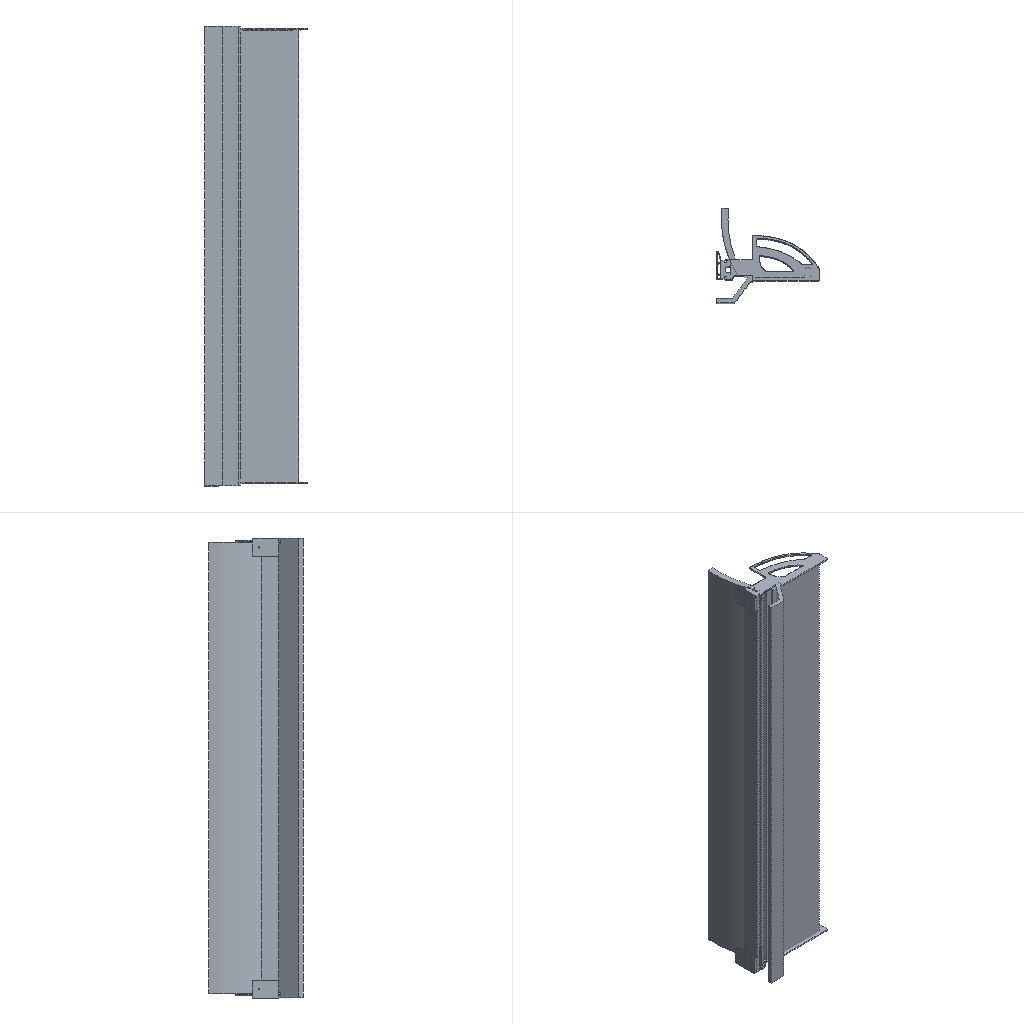Simulation study | ansys workbench
Set-up summary:
category,name,step,type,value,unit,region
solver,ansys_workbench
units,mm-N-s-tonne (MPa),,stated,"/units,MPA"
analysis,LS1,,static
load_step,LS1,LS1,static,nsubst=1; time=1
mesh,nodes,,,334220
mesh,elements,,,128560
element_type,SOLID187,,,74774
element_type,SOLID186,,,34803
element_type,SURF154,,,11977
element_type,TARGE170,,,3503
element_type,CONTA174,,,3503
material,Structural Steel,,E,200000,tonne s^-2 mm^-1
material,Structural Steel,,nu,0.3
material,Structural Steel,,density,7.85e-09,tonne mm^-3
material,Structural Steel,,conductivity,60.5,tonne mm s^-3 C^-1
material,Structural Steel,,specific_heat,4.34e+08,mm^2 s^-2 C^-1
material,Structural Steel,,cte,1.2e-05,C^-1
material,Structural Steel,,permeability,10000
material,Structural Steel,,resistivity,0.00017,ohm mm
load,Define Force Using Surface Effect Elements,LS1,surface-effect pres face 2,-0.009735,,SURF154 #25
load,Define Force Using Surface Effect Elements,LS1,surface-effect pres face 1,-0.008186,,SURF154 #26
bc,Fixed Supports,model,fixed,[dofs=ALL],,_FIXEDSU
contact,Contact Region,,bonded (always),element=CONTA174
contact,Contact Region 2,,bonded (always),element=CONTA174
contact,Contact Region 3,,bonded (always),element=CONTA174
contact,Contact Region 4,,bonded (always),element=CONTA174
contact,Contact Region 5,,bonded (always),element=CONTA174
contact,Contact Region 6,,bonded (always),element=CONTA174
contact,Contact Region 7,,bonded (always),element=CONTA174
contact,Contact Region 8,,bonded (always),element=CONTA174
contact,Contact Region 9,,bonded (always),element=CONTA174
named_set,______,,node,840
named_set,_FIXEDSU,,node,17233
Ansys APDL input file, long lists of numbers shortened:
/batch
/config,noeldb,1     ! force off writing results to database
*get,_wallstrt,active,,time,wall
! ANSYS input file written by Workbench version 2022 R1
! File used for geometry attach:
/title,wbnew--____ (B5)
! ****** Begin Custom Load Command Snippet ******
/COM, ACT Extensions:
/COM,     LSDYNA, 2021.1
/COM,
! ****** End   Custom Load Command Snippet ******
*DIM,_wb_ProjectScratch_dir,string,248
_wb_ProjectScratch_dir(1) = ''
*DIM,_wb_SolverFiles_dir,string,248
_wb_SolverFiles_dir(1) = ''
*DIM,_wb_userfiles_dir,string,248
_wb_userfiles_dir(1) = ''
/com,--- Data in consistent NMM units. See Solving Units in the help system for more information.
/units,MPA
/nopr
/wb,file,start              !  signify a WB generated input file
/prep7
! Turn off shape checking because checks already performed inside WB mesher.
! See help system for more information.
SHPP,OFF,,NOWARN
/nolist
etcon,set             ! allow ANSYS to choose best KEYOP's for 180x elements, resets any applicable keyopt to MAPDL defaults
/com,*********** Nodes for the whole assembly ***********
nblock,3,,367642
(1i9,3e20.9e3)
        1    -2.456414230E+02    -1.995121614E+02    -2.244930474E+03
! (334219 more lines like these left out)
-1
/wb,elem,start            !  set before creation of elements
/com,*********** Elements for Body 1 "____|__2" ***********
et,1,187
eblock,19,solid,,9964
(19i9)
        1        1        1        1        0        0        0        0       10        0    44768   216403   217349   219644   219638   220099   227118   220105   220104
! (19927 more lines like these left out)
-1
/com,*********** Elements for Body 2 "____|__2" ***********
et,2,187
eblock,19,solid,,54846
(19i9)
        2        2        2        2        0        0        0        0       10        0    54732   237393   251383   247928   251349   262974   322040   262970   262973
! (109691 more lines like these left out)
-1
/com,*********** Elements for Body 3 "____|__2[2]" ***********
et,3,187
eblock,19,solid,,9964
(19i9)
        3        3        3        3        0        0        0        0       10        0    34804   196829   197775   200070   200064   200525   207544   200531   200530
! (19927 more lines like these left out)
-1
/com,*********** Elements for Body 4 "__|__-__1" ***********
et,4,186
keyo,4,2,1          ! set full integration on SOLID186
eblock,19,solid,,19488
(19i9)
        4        4        4        4        0        0        0        0       20        0    15316    96729   117001   123497   123624   109656   123465   123466   123656
! (38975 more lines like these left out)
-1
/com,*********** Elements for Body 5 "__|__1" ***********
et,5,186
keyo,5,2,1          ! set full integration on SOLID186
eblock,19,solid,,9135
(19i9)
        5        5        5        5        0        0        0        0       20        0     6181    39485    39493    39488    39486    41715    41707    41712    41714
! (18269 more lines like these left out)
-1
/com,*********** Elements for Body 6 "___|__-__1" ***********
et,6,186
keyo,6,2,1          ! set full integration on SOLID186
eblock,19,solid,,6180
(19i9)
        6        6        6        6        0        0        0        0       20        0        1        1     8717     8502     7059     1648    10962     8501     8500
! (12359 more lines like these left out)
-1
/wb,elem,end               !  done creating elements
/com,*********** Send User Defined Coordinate System(s) ***********
csys,0
toffst,273.15,  ! Temperature offset from absolute zero
/com,*********** Set Reference Temperature ***********
tref,22.
/wb,mat,start              !  starting to send materials
/com,*********** Send Materials ***********
Temperature = 'TEMP' ! Temperature
MP,DENS,1,7.85e-09,	! tonne mm^-3
MP,ALPX,1,1.2e-05,	! C^-1
MP,C,1,434000000,	! mm^2 s^-2 C^-1
MP,KXX,1,60.5,	! tonne mm s^-3 C^-1
MP,RSVX,1,0.00017,	! ohm mm
MP,EX,1,200000,	! tonne s^-2 mm^-1
MP,NUXY,1,0.3,
MP,MURX,1,10000,
Temperature = 'TEMP' ! Temperature
MP,DENS,2,7.85e-09,	! tonne mm^-3
MP,ALPX,2,1.2e-05,	! C^-1
MP,C,2,434000000,	! mm^2 s^-2 C^-1
MP,KXX,2,60.5,	! tonne mm s^-3 C^-1
MP,RSVX,2,0.00017,	! ohm mm
MP,EX,2,200000,	! tonne s^-2 mm^-1
MP,NUXY,2,0.3,
MP,MURX,2,10000,
Temperature = 'TEMP' ! Temperature
MP,DENS,3,7.85e-09,	! tonne mm^-3
MP,ALPX,3,1.2e-05,	! C^-1
MP,C,3,434000000,	! mm^2 s^-2 C^-1
MP,KXX,3,60.5,	! tonne mm s^-3 C^-1
MP,RSVX,3,0.00017,	! ohm mm
MP,EX,3,200000,	! tonne s^-2 mm^-1
MP,NUXY,3,0.3,
MP,MURX,3,10000,
Temperature = 'TEMP' ! Temperature
MP,DENS,4,7.85e-09,	! tonne mm^-3
MP,ALPX,4,1.2e-05,	! C^-1
MP,C,4,434000000,	! mm^2 s^-2 C^-1
MP,KXX,4,60.5,	! tonne mm s^-3 C^-1
MP,RSVX,4,0.00017,	! ohm mm
MP,EX,4,200000,	! tonne s^-2 mm^-1
MP,NUXY,4,0.3,
MP,MURX,4,10000,
Temperature = 'TEMP' ! Temperature
MP,DENS,5,7.85e-09,	! tonne mm^-3
MP,ALPX,5,1.2e-05,	! C^-1
MP,C,5,434000000,	! mm^2 s^-2 C^-1
MP,KXX,5,60.5,	! tonne mm s^-3 C^-1
MP,RSVX,5,0.00017,	! ohm mm
MP,EX,5,200000,	! tonne s^-2 mm^-1
MP,NUXY,5,0.3,
MP,MURX,5,10000,
Temperature = 'TEMP' ! Temperature
MP,DENS,6,7.85e-09,	! tonne mm^-3
MP,ALPX,6,1.2e-05,	! C^-1
MP,C,6,434000000,	! mm^2 s^-2 C^-1
MP,KXX,6,60.5,	! tonne mm s^-3 C^-1
MP,RSVX,6,0.00017,	! ohm mm
MP,EX,6,200000,	! tonne s^-2 mm^-1
MP,NUXY,6,0.3,
MP,MURX,6,10000,
/wb,mat,end                !  done sending materials
!************************* Model Summary ********************
!____|__2,	结构钢,	matid,	1
!____|__2,	结构钢,	matid,	2
!____|__2[2],	结构钢,	matid,	3
!__|__-__1,	结构钢,	matid,	4
!__|__1,	结构钢,	matid,	5
!___|__-__1,	结构钢,	matid,	6
!************************* End Model Summary ********************
! get the diagonal of the bounding box. Needed later for other things
*get,_xmin,node,,mnloc,x
*get,_ymin,node,,mnloc,y
*get,_zmin,node,,mnloc,z
*get,_xmax,node,,mxloc,x
*get,_ymax,node,,mxloc,y
*get,_zmax,node,,mxloc,z
_ASMDIAG=(_xmax-_xmin)*(_xmax-_xmin)+(_ymax-_ymin)*(_ymax-_ymin)+(_zmax-_zmin)*(_zmax-_zmin)
_ASMDIAG=SQRT(_ASMDIAG)
/wb,contact,start          !  starting to send contact
/com,*********** Create Contact "接触区域" ***********
/com,            Real Constant Set For Above Contact Is 8 & 7
*set,tid,8
*set,cid,7
r,tid
r,cid
et,tid,170
et,cid,174
eblock,10,,,210
(15i9)
   182904        8        8        8        0   216357   217399   216360   216360   219805   219825   216360   219802
! (209 more lines like these left out)
-1
eblock,10,,,210
(15i9)
   183114        7        7        7        0   216357   217399   216360   216360   219805   219825   216360   219802
! (209 more lines like these left out)
-1
eblock,10,,,188
(15i9)
   183324        7        8        7        0   238612   243412   238618   238618   271681   271714   238618   271680
! (187 more lines like these left out)
-1
eblock,10,,,188
(15i9)
   183512        8        7        8        0   238612   243412   238618   238618   271681   271714   238618   271680
! (187 more lines like these left out)
-1
keyo,cid,8,2               ! auto create asymmetric contact (from Program Controlled setting)
keyo,cid,10,0              ! adjust contact stiffness each NR iteration (from Program Controlled setting)
keyo,cid,12,5              ! bonded always
keyo,cid,18,1              ! small sliding turned on by application
keyo,cid,2,0               ! augmented Lagrange (from Program Controlled setting)
keyo,cid,4,0               ! on Gauss point (from Program Controlled setting)
keyo,cid,9,1               ! ignore initial gaps/penetration
keyo,cid,7,0               ! No Prediction
rmod,tid,3,10.      ! FKN
rmod,tid,5,0.       ! ICONT
rmod,tid,6,0.       ! PINB
rmod,tid,10,0.      ! CNOF
rmod,tid,12,0.      ! FKT
rmod,tid,36,41      ! WB DSID
rmod,cid,3,10.      ! FKN
rmod,cid,5,0.       ! ICONT
rmod,cid,6,0.       ! PINB
rmod,cid,10,0.      ! CNOF
rmod,cid,12,0.      ! FKT
rmod,cid,36,41      ! WB DSID
/com,*********** Create Contact "接触区域 2" ***********
/com,            Real Constant Set For Above Contact Is 10 & 9
*set,tid,10
*set,cid,9
r,tid
r,cid
et,tid,170
et,cid,174
eblock,10,,,109
(15i9)
   183700       10       10       10        0   218830   219036   218891   218891   233905   234246   218891   233902
! (108 more lines like these left out)
-1
eblock,10,,,109
(15i9)
   183809        9        9        9        0   218830   219036   218891   218891   233905   234246   218891   233902
! (108 more lines like these left out)
-1
eblock,10,,,30
(15i9)
   183918        9       10        9        0   123655   123593   116939   116938   196669   183568   183565   183566
! (29 more lines like these left out)
-1
eblock,10,,,30
(15i9)
   183948       10        9       10        0   123655   123593   116939   116938   196669   183568   183565   183566
! (29 more lines like these left out)
-1
keyo,cid,8,2               ! auto create asymmetric contact (from Program Controlled setting)
keyo,cid,10,0              ! adjust contact stiffness each NR iteration (from Program Controlled setting)
keyo,cid,12,5              ! bonded always
keyo,cid,18,1              ! small sliding turned on by application
keyo,cid,2,0               ! augmented Lagrange (from Program Controlled setting)
keyo,cid,4,0               ! on Gauss point (from Program Controlled setting)
keyo,cid,9,1               ! ignore initial gaps/penetration
keyo,cid,7,0               ! No Prediction
rmod,tid,3,10.      ! FKN
rmod,tid,5,0.       ! ICONT
rmod,tid,6,0.       ! PINB
rmod,tid,10,0.      ! CNOF
rmod,tid,12,0.      ! FKT
rmod,tid,36,44      ! WB DSID
rmod,cid,3,10.      ! FKN
rmod,cid,5,0.       ! ICONT
rmod,cid,6,0.       ! PINB
rmod,cid,10,0.      ! CNOF
rmod,cid,12,0.      ! FKT
rmod,cid,36,44      ! WB DSID
/com,*********** Create Contact "接触区域 3" ***********
/com,            Real Constant Set For Above Contact Is 12 & 11
*set,tid,12
*set,cid,11
r,tid
r,cid
et,tid,170
et,cid,174
eblock,10,,,422
(15i9)
   183978       12       12       12        0   218902   219011   218909   218909   234298   234321   218909   234296
! (421 more lines like these left out)
-1
eblock,10,,,422
(15i9)
   184400       11       11       11        0   218902   219011   218909   218909   234298   234321   218909   234296
! (421 more lines like these left out)
-1
eblock,10,,,45
(15i9)
   184822       11       12       11        0    41721    41719    41720    41720    63525    63524    41720    63527
! (44 more lines like these left out)
-1
eblock,10,,,45
(15i9)
   184867       12       11       12        0    41721    41719    41720    41720    63525    63524    41720    63527
! (44 more lines like these left out)
-1
keyo,cid,8,2               ! auto create asymmetric contact (from Program Controlled setting)
keyo,cid,10,0              ! adjust contact stiffness each NR iteration (from Program Controlled setting)
keyo,cid,12,5              ! bonded always
keyo,cid,18,1              ! small sliding turned on by application
keyo,cid,2,0               ! augmented Lagrange (from Program Controlled setting)
keyo,cid,4,0               ! on Gauss point (from Program Controlled setting)
keyo,cid,9,1               ! ignore initial gaps/penetration
keyo,cid,7,0               ! No Prediction
rmod,tid,3,10.      ! FKN
rmod,tid,5,0.       ! ICONT
rmod,tid,6,0.       ! PINB
rmod,tid,10,0.      ! CNOF
rmod,tid,12,0.      ! FKT
rmod,tid,36,47      ! WB DSID
rmod,cid,3,10.      ! FKN
rmod,cid,5,0.       ! ICONT
rmod,cid,6,0.       ! PINB
rmod,cid,10,0.      ! CNOF
rmod,cid,12,0.      ! FKT
rmod,cid,36,47      ! WB DSID
/com,*********** Create Contact "接触区域 4" ***********
/com,            Real Constant Set For Above Contact Is 14 & 13
*set,tid,14
*set,cid,13
r,tid
r,cid
et,tid,170
et,cid,174
eblock,10,,,44
(15i9)
   184912       14       14       14        0   216522   217504   216520   216520   220941   220930   216520   220925
! (43 more lines like these left out)
-1
eblock,10,,,44
(15i9)
   184956       13       13       13        0   216522   217504   216520   216520   220941   220930   216520   220925
! (43 more lines like these left out)
-1
eblock,10,,,6
(15i9)
   185000       13       14       13        0     1701     1703     2320     1700    18310    18314    18308    18307
   185001       13       14       13        0     1702     2114     1703     1701    18311    18313    18310    18309
   185002       13       14       13        0     1703     1704     2319     2320    18312    18317    19748    18314
   185003       13       14       13        0     2114     2113     1704     1703    19337    18316    18312    18313
   185004       13       14       13        0     1704     1705     2318     2319    18315    18320    19746    18317
   185005       13       14       13        0     2113     2112     1705     1704    19335    18319    18315    18316
-1
eblock,10,,,6
(15i9)
   185006       14       13       14        0     1701     1703     2320     1700    18310    18314    18308    18307
   185007       14       13       14        0     1702     2114     1703     1701    18311    18313    18310    18309
   185008       14       13       14        0     1703     1704     2319     2320    18312    18317    19748    18314
   185009       14       13       14        0     2114     2113     1704     1703    19337    18316    18312    18313
   185010       14       13       14        0     1704     1705     2318     2319    18315    18320    19746    18317
   185011       14       13       14        0     2113     2112     1705     1704    19335    18319    18315    18316
-1
keyo,cid,8,2               ! auto create asymmetric contact (from Program Controlled setting)
keyo,cid,10,0              ! adjust contact stiffness each NR iteration (from Program Controlled setting)
keyo,cid,12,5              ! bonded always
keyo,cid,18,1              ! small sliding turned on by application
keyo,cid,2,0               ! augmented Lagrange (from Program Controlled setting)
keyo,cid,4,0               ! on Gauss point (from Program Controlled setting)
keyo,cid,9,1               ! ignore initial gaps/penetration
keyo,cid,7,0               ! No Prediction
rmod,tid,3,10.      ! FKN
rmod,tid,5,0.       ! ICONT
rmod,tid,6,0.       ! PINB
rmod,tid,10,0.      ! CNOF
rmod,tid,12,0.      ! FKT
rmod,tid,36,50      ! WB DSID
rmod,cid,3,10.      ! FKN
rmod,cid,5,0.       ! ICONT
rmod,cid,6,0.       ! PINB
rmod,cid,10,0.      ! CNOF
rmod,cid,12,0.      ! FKT
rmod,cid,36,50      ! WB DSID
/com,*********** Create Contact "接触区域 5" ***********
/com,            Real Constant Set For Above Contact Is 16 & 15
*set,tid,16
*set,cid,15
r,tid
r,cid
et,tid,170
et,cid,174
eblock,10,,,186
(15i9)
   185012       16       16       16        0   238203   238205   238410   238410   268770   268781   238410   268771
! (185 more lines like these left out)
-1
eblock,10,,,186
(15i9)
   185198       15       15       15        0   238203   238205   238410   238410   268770   268781   238410   268771
! (185 more lines like these left out)
-1
eblock,10,,,210
(15i9)
   185384       15       16       15        0   196787   196803   196810   196810   200257   200367   196810   200258
! (209 more lines like these left out)
-1
eblock,10,,,210
(15i9)
   185594       16       15       16        0   196787   196803   196810   196810   200257   200367   196810   200258
! (209 more lines like these left out)
-1
keyo,cid,8,2               ! auto create asymmetric contact (from Program Controlled setting)
keyo,cid,10,0              ! adjust contact stiffness each NR iteration (from Program Controlled setting)
keyo,cid,12,5              ! bonded always
keyo,cid,18,1              ! small sliding turned on by application
keyo,cid,2,0               ! augmented Lagrange (from Program Controlled setting)
keyo,cid,4,0               ! on Gauss point (from Program Controlled setting)
keyo,cid,9,1               ! ignore initial gaps/penetration
keyo,cid,7,0               ! No Prediction
rmod,tid,3,10.      ! FKN
rmod,tid,5,0.       ! ICONT
rmod,tid,6,0.       ! PINB
rmod,tid,10,0.      ! CNOF
rmod,tid,12,0.      ! FKT
rmod,tid,36,53      ! WB DSID
rmod,cid,3,10.      ! FKN
rmod,cid,5,0.       ! ICONT
rmod,cid,6,0.       ! PINB
rmod,cid,10,0.      ! CNOF
rmod,cid,12,0.      ! FKT
rmod,cid,36,53      ! WB DSID
/com,*********** Create Contact "接触区域 6" ***********
/com,            Real Constant Set For Above Contact Is 18 & 17
*set,tid,18
*set,cid,17
r,tid
r,cid
et,tid,170
et,cid,174
eblock,10,,,95
(15i9)
   185804       18       18       18        0   198886   198939   199065   199065   211719   212247   199065   211722
! (94 more lines like these left out)
-1
eblock,10,,,95
(15i9)
   185899       17       17       17        0   198886   198939   199065   199065   211719   212247   199065   211722
! (94 more lines like these left out)
-1
eblock,10,,,30
(15i9)
   185994       17       18       17        0   123550   123551   116978   116979   196615   183645   183644   183647
! (29 more lines like these left out)
-1
eblock,10,,,30
(15i9)
   186024       18       17       18        0   123550   123551   116978   116979   196615   183645   183644   183647
! (29 more lines like these left out)
-1
keyo,cid,8,2               ! auto create asymmetric contact (from Program Controlled setting)
keyo,cid,10,0              ! adjust contact stiffness each NR iteration (from Program Controlled setting)
keyo,cid,12,5              ! bonded always
keyo,cid,18,1              ! small sliding turned on by application
keyo,cid,2,0               ! augmented Lagrange (from Program Controlled setting)
keyo,cid,4,0               ! on Gauss point (from Program Controlled setting)
keyo,cid,9,1               ! ignore initial gaps/penetration
keyo,cid,7,0               ! No Prediction
rmod,tid,3,10.      ! FKN
rmod,tid,5,0.       ! ICONT
rmod,tid,6,0.       ! PINB
rmod,tid,10,0.      ! CNOF
rmod,tid,12,0.      ! FKT
rmod,tid,36,56      ! WB DSID
rmod,cid,3,10.      ! FKN
rmod,cid,5,0.       ! ICONT
rmod,cid,6,0.       ! PINB
rmod,cid,10,0.      ! CNOF
rmod,cid,12,0.      ! FKT
rmod,cid,36,56      ! WB DSID
/com,*********** Create Contact "接触区域 7" ***********
/com,            Real Constant Set For Above Contact Is 20 & 19
*set,tid,20
*set,cid,19
r,tid
r,cid
et,tid,170
et,cid,174
eblock,10,,,406
(15i9)
   186054       20       20       20        0   198991   199061   199033   199033   212711   213012   199033   212710
! (405 more lines like these left out)
-1
eblock,10,,,406
(15i9)
   186460       19       19       19        0   198991   199061   199033   199033   212711   213012   199033   212710
! (405 more lines like these left out)
-1
eblock,10,,,45
(15i9)
   186866       19       20       19        0    41712    41713    41714    41714    63507    63510    41714    63508
! (44 more lines like these left out)
-1
eblock,10,,,45
(15i9)
   186911       20       19       20        0    41712    41713    41714    41714    63507    63510    41714    63508
! (44 more lines like these left out)
-1
keyo,cid,8,2               ! auto create asymmetric contact (from Program Controlled setting)
keyo,cid,10,0              ! adjust contact stiffness each NR iteration (from Program Controlled setting)
keyo,cid,12,5              ! bonded always
keyo,cid,18,1              ! small sliding turned on by application
keyo,cid,2,0               ! augmented Lagrange (from Program Controlled setting)
keyo,cid,4,0               ! on Gauss point (from Program Controlled setting)
keyo,cid,9,1               ! ignore initial gaps/penetration
keyo,cid,7,0               ! No Prediction
rmod,tid,3,10.      ! FKN
rmod,tid,5,0.       ! ICONT
rmod,tid,6,0.       ! PINB
rmod,tid,10,0.      ! CNOF
rmod,tid,12,0.      ! FKT
rmod,tid,36,59      ! WB DSID
rmod,cid,3,10.      ! FKN
rmod,cid,5,0.       ! ICONT
rmod,cid,6,0.       ! PINB
rmod,cid,10,0.      ! CNOF
rmod,cid,12,0.      ! FKT
rmod,cid,36,59      ! WB DSID
/com,*********** Create Contact "接触区域 8" ***********
/com,            Real Constant Set For Above Contact Is 22 & 21
*set,tid,22
*set,cid,21
r,tid
r,cid
et,tid,170
et,cid,174
eblock,10,,,44
(15i9)
   186956       22       22       22        0   196948   197930   196946   196946   201367   201356   196946   201351
! (43 more lines like these left out)
-1
eblock,10,,,44
(15i9)
   187000       21       21       21        0   196948   197930   196946   196946   201367   201356   196946   201351
! (43 more lines like these left out)
-1
eblock,10,,,6
(15i9)
   187044       21       22       21        0     1905     1906     2117     2118    18918    18923    19344    18920
   187045       21       22       21        0     1912     1911     1906     1905    18933    18922    18918    18919
   187046       21       22       21        0     1906     1907     2116     2117    18921    18926    19342    18923
   187047       21       22       21        0     1911     1910     1907     1906    18931    18925    18921    18922
   187048       21       22       21        0     1907     1908     2115     2116    18924    18928    19340    18926
   187049       21       22       21        0     1910     1909     1908     1907    18929    18927    18924    18925
-1
eblock,10,,,6
(15i9)
   187050       22       21       22        0     1905     1906     2117     2118    18918    18923    19344    18920
   187051       22       21       22        0     1912     1911     1906     1905    18933    18922    18918    18919
   187052       22       21       22        0     1906     1907     2116     2117    18921    18926    19342    18923
   187053       22       21       22        0     1911     1910     1907     1906    18931    18925    18921    18922
   187054       22       21       22        0     1907     1908     2115     2116    18924    18928    19340    18926
   187055       22       21       22        0     1910     1909     1908     1907    18929    18927    18924    18925
-1
keyo,cid,8,2               ! auto create asymmetric contact (from Program Controlled setting)
keyo,cid,10,0              ! adjust contact stiffness each NR iteration (from Program Controlled setting)
keyo,cid,12,5              ! bonded always
keyo,cid,18,1              ! small sliding turned on by application
keyo,cid,2,0               ! augmented Lagrange (from Program Controlled setting)
keyo,cid,4,0               ! on Gauss point (from Program Controlled setting)
keyo,cid,9,1               ! ignore initial gaps/penetration
keyo,cid,7,0               ! No Prediction
rmod,tid,3,10.      ! FKN
rmod,tid,5,0.       ! ICONT
rmod,tid,6,0.       ! PINB
rmod,tid,10,0.      ! CNOF
rmod,tid,12,0.      ! FKT
rmod,tid,36,62      ! WB DSID
rmod,cid,3,10.      ! FKN
rmod,cid,5,0.       ! ICONT
rmod,cid,6,0.       ! PINB
rmod,cid,10,0.      ! CNOF
rmod,cid,12,0.      ! FKT
rmod,cid,36,62      ! WB DSID
/com,*********** Create Contact "接触区域 9" ***********
/com,            Real Constant Set For Above Contact Is 24 & 23
*set,tid,24
*set,cid,23
r,tid
r,cid
et,tid,170
et,cid,174
eblock,10,,,1015
(15i9)
   187056       24       24       24        0    48315    48316    53972    53971    82625    82630    93891    82627
! (1014 more lines like these left out)
-1
eblock,10,,,1015
(15i9)
   188071       23       23       23        0    48315    48316    53972    53971    82625    82630    93891    82627
! (1014 more lines like these left out)
-1
eblock,10,,,412
(15i9)
   189086       23       24       23        0     2528     2321     2526     2527    19753    19752    20161    20162
! (411 more lines like these left out)
-1
eblock,10,,,412
(15i9)
   189498       24       23       24        0     2528     2321     2526     2527    19753    19752    20161    20162
! (411 more lines like these left out)
-1
keyo,cid,8,2               ! auto create asymmetric contact (from Program Controlled setting)
keyo,cid,10,0              ! adjust contact stiffness each NR iteration (from Program Controlled setting)
keyo,cid,12,5              ! bonded always
keyo,cid,18,1              ! small sliding turned on by application
keyo,cid,2,0               ! augmented Lagrange (from Program Controlled setting)
keyo,cid,4,0               ! on Gauss point (from Program Controlled setting)
keyo,cid,9,1               ! ignore initial gaps/penetration
keyo,cid,7,0               ! No Prediction
rmod,tid,3,10.      ! FKN
rmod,tid,5,0.       ! ICONT
rmod,tid,6,0.       ! PINB
rmod,tid,10,0.      ! CNOF
rmod,tid,12,0.      ! FKT
rmod,tid,36,65      ! WB DSID
rmod,cid,3,10.      ! FKN
rmod,cid,5,0.       ! ICONT
rmod,cid,6,0.       ! PINB
rmod,cid,10,0.      ! CNOF
rmod,cid,12,0.      ! FKT
rmod,cid,36,65      ! WB DSID
nsel,all
esel,all
/wb,contact,end            !  done creating contacts
/com,*********** Send Named Selection as Node Component ***********
CMBLOCK,______  ,NODE,      840
(8i10)
    196779    196780    196781    196782    196783    196784    196785    196786
! (104 more lines like these left out)
/golist
/wb,load,start             !  starting to send loads
/com,*********** Fixed Supports ***********
CMBLOCK,_FIXEDSU,NODE,    17233
(8i10)
      1669      1670      1671      1672      1673      1674      1675      1676
! (2154 more lines like these left out)
cmsel,s,_FIXEDSU
d,all,all
nsel,all
/com,*********** Define Force Using Surface Effect Elements ***********
local,12,0,0.,0.,0.,0.,0.,0.
csys,0
et,25,154
eblock,10,,,5481
(15i9)
   189910       25       25       25       12    47478    41796    47073    47479    63711    63710    79717    80729
! (5480 more lines like these left out)
-1
esel,s,type,,25
keyop,25,2,1                ! Apply load in local coordinate system
keyop,25,7,1                ! Use original area so load is constant in large deformation
esel,all
/com,*********** Define Force Using Surface Effect Elements ***********
local,13,0,0.,0.,0.,0.,0.,0.
csys,0
et,26,154
eblock,10,,,6496
(15i9)
   195391       26       26       26       13   123465   117001   123497   123466   183691   183692   196449   196448
! (6495 more lines like these left out)
-1
esel,s,type,,26
keyop,26,2,1                ! Apply load in local coordinate system
keyop,26,7,1                ! Use original area so load is constant in large deformation
esel,all
/gst,on,on
fini
*get,_numnode,node,0,count
*get,_numelem,elem,0,count
*get, _MAXELEMNUM, elem, 0, NUM, MAX
*get, _MAXNODENUM, node, 0, NUM, MAX
*get, _MAXELEMTYPE, etyp, 0, NUM, MAX
*get, _MAXREALCONST, real, 0, NUM, MAX
/go
/wb,load,end               !  done creating loads
/com,--- Number of total nodes = %_numnode%
/com,--- Number of contact elements = 18983
/com,--- Number of spring elements = 0
/com,--- Number of bearing elements = 0
/com,--- Number of solid elements = 109577
/com,--- Number of condensed parts = 0
/com,--- Number of total elements = %_numelem%
*get,_wallbsol,active,,time,wall
/com,****************************************************************************
/com,*************************    SOLUTION       ********************************
/com,****************************************************************************
/solu
antype,0                   ! static analysis
_thickRatio=0.5     ! Ratio of thick parts in the model
eqsl,sparse,,,,,1
cntr,print,1               ! print out contact info and also make no initial contact an error
dmpoption,emat,no             ! Don't combine emat file for DANSYS
dmpoption,esav,no             ! Don't combine esav file for DANSYS
nldiag,cont,iter           ! print out contact info each equilibrium iteration
rescontrol,,none                 ! Do not keep any restart files
/com,****************************************************
/com,******************* SOLVE FOR LS 1 OF 1 ****************
esel,s,type,,25
nsle
sfe,all,1,pres,1,0.
sfe,all,2,pres,1,-9.73503147416359e-003
sfe,all,3,pres,1,0.
esel,s,type,,26
nsle
sfe,all,1,pres,1,-8.1857805763087e-003
sfe,all,2,pres,1,0.
sfe,all,3,pres,1,0.
nsel,all
esel,all
/nopr
/gopr
nsub,1,1,1
time,1.
outres,erase
outres,all,none
outres,nsol,all,
outres,rsol,all
outres,eangl,all
outres,etmp,all
outres,veng,all
outres,strs,all,
outres,epel,all,
outres,eppl,all,
outres,cont,all,
! *********** WB SOLVE COMMAND ***********
! check interactive state
*get,ANSINTER_,active,,int
*if,ANSINTER_,ne,0,then
/eof
*endif
solve
/com *************** Write FE CONNECTORS *********
CEWRITE,file,ce,,INTE
/com,****************************************************
/com,*************** FINISHED SOLVE FOR LS 1 *************
*get,_wallasol,active,,time,wall
/nopr
*get,_numnode,node,0,count
*get,_numelem,elem,0,count
*get, _MAXELEMNUM, elem, 0, NUM, MAX
*get, _MAXNODENUM, node, 0, NUM, MAX,,,INTERNAL
*get, _MAXELEMTYPE, etyp, 0, NUM, MAX
*get, _MAXREALCONST, real, 0, NUM, MAX
/gopr
/post1
xmlo,ENCODING,ISO-8859-1
xmlo,parm
/xml,parm,xml
fini
/gopr
*get,_walldone,active,,time,wall
_preptime=(_wallbsol-_wallstrt)*3600
_solvtime=(_wallasol-_wallbsol)*3600
_posttime=(_walldone-_wallasol)*3600
_totaltim=(_walldone-_wallstrt)*3600
*get,_dlbratio,active,0,solu,dlbr
*get,_combtime,active,0,solu,comb
*get,_ssmode,active,0,solu,ssmm
*get,_ndofs,active,0,solu,ndof
*get,_sol_end_time,active,0,set,time
*if,_sol_end_time,eq,1.,then
/fclean				!clean distributed files
*endif
/com,--- Total number of nodes = %_numnode%
/com,--- Total number of elements = %_numelem%
/com,--- Element load balance ratio = %_dlbratio%
/com,--- Time to combine distributed files = %_combtime%
/com,--- Sparse memory mode = %_ssmode%
/com,--- Number of DOF = %_ndofs%
/wb,file,end               ! done with WB generated input
Results summary:
result,analyses[0].index,,,1
result,analyses[0].system,,,SYS
result,analyses[0].deck,,,deck.dat
result,analyses[0].solve_status,,,completed
result,analyses[0].analysis_type,,,static
result,analyses[0].physics,,,mechanical
result,analyses[0].unit_system,,,"NMM: mm, ton, N, s, mV, mA, degC"
result,analyses[0].n_sets,,,1
result,analyses[0].load_steps[0].set,set=1,,1
result,analyses[0].load_steps[0].time_or_freq,set=1,,1
result,analyses[0].load_steps[0].max_displacement_magnitude,set=1,,0.1589
result,analyses[0].load_steps[0].max_von_mises_nodal,set=1,,16.938
result,analyses[0].load_steps[0].reaction_force_sum_xyz[1],set=1,,5200
result,analyses[0].load_steps[0].reaction_force_sum_xyz[2],set=1,,5320
result,analyses[0].load_steps[0].reaction_force_sum_xyz[3],set=1,,9.85717e-05